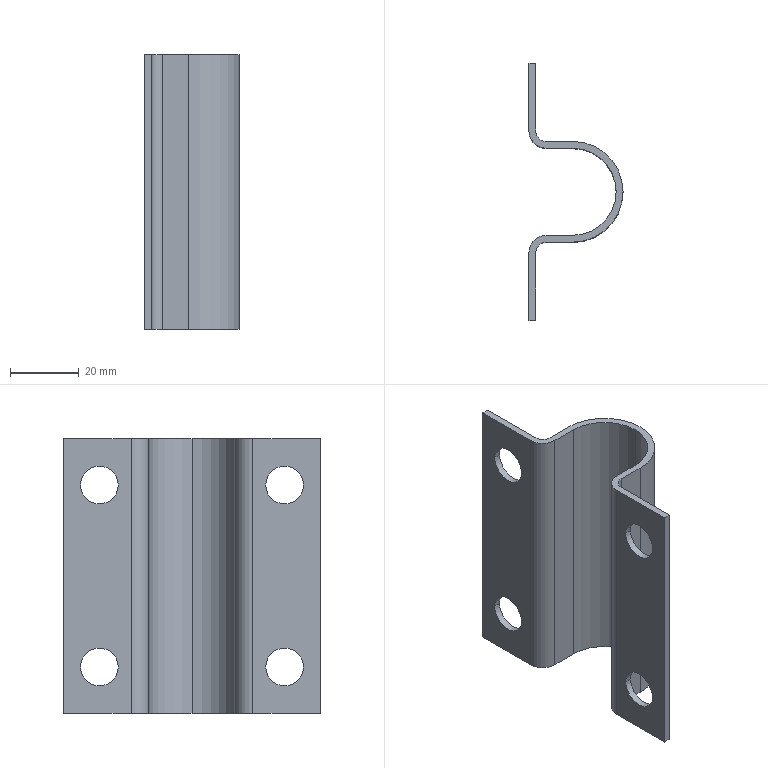Part | STEP file | 750031837 | 1 solid | 28 faces | box 27.4 x 75 x 80 mm | volume 16937 mm3 | cylinder 16 | plane 12 | commonest cylinder face diameters 11 x8 6 x2 10 x2 25.4 x2 29.4 x2
STEP:
#1=CARTESIAN_POINT('',(12.7,-14.7,0.));
#2=VERTEX_POINT('',#1);
#3=CARTESIAN_POINT('',(27.4,0.,0.));
#4=VERTEX_POINT('',#3);
#5=CARTESIAN_POINT('',(12.7,0.,0.));
#6=DIRECTION('',(0.,0.,1.));
#7=DIRECTION('',(1.,0.,0.));
#8=AXIS2_PLACEMENT_3D('',#5,#6,#7);
#9=CIRCLE('',#8,14.7);
#10=EDGE_CURVE('',#2,#4,#9,.T.);
#11=ORIENTED_EDGE('',*,*,#10,.T.);
#12=CARTESIAN_POINT('',(27.4,0.,80.));
#13=VERTEX_POINT('',#12);
#14=CARTESIAN_POINT('',(27.4,0.,0.));
#15=DIRECTION('',(0.,0.,1.));
#16=VECTOR('',#15,1000.);
#17=LINE('',#14,#16);
#18=EDGE_CURVE('',#4,#13,#17,.T.);
#19=ORIENTED_EDGE('',*,*,#18,.T.);
#20=CARTESIAN_POINT('',(12.7,-14.7,80.));
#21=VERTEX_POINT('',#20);
#22=CARTESIAN_POINT('',(12.7,0.,80.));
#23=DIRECTION('',(0.,0.,-1.));
#24=DIRECTION('',(1.,0.,0.));
#25=AXIS2_PLACEMENT_3D('',#22,#23,#24);
#26=CIRCLE('',#25,14.7);
#27=EDGE_CURVE('',#13,#21,#26,.T.);
#28=ORIENTED_EDGE('',*,*,#27,.T.);
#29=CARTESIAN_POINT('',(12.7,-14.7,0.));
#30=DIRECTION('',(0.,0.,-1.));
#31=VECTOR('',#30,1000.);
#32=LINE('',#29,#31);
#33=EDGE_CURVE('',#21,#2,#32,.T.);
#34=ORIENTED_EDGE('',*,*,#33,.T.);
#35=EDGE_LOOP('',(#11,#19,#28,#34));
#36=FACE_OUTER_BOUND('',#35,.T.);
#37=CARTESIAN_POINT('',(12.7,0.,0.));
#38=DIRECTION('',(0.,0.,1.));
#39=DIRECTION('',(1.,0.,0.));
#40=AXIS2_PLACEMENT_3D('',#37,#38,#39);
#41=CYLINDRICAL_SURFACE('',#40,14.7);
#42=ADVANCED_FACE('',(#36),#41,.T.);
#43=CARTESIAN_POINT('',(25.4,0.,0.));
#44=VERTEX_POINT('',#43);
#45=CARTESIAN_POINT('',(12.7,12.7,0.));
#46=VERTEX_POINT('',#45);
#47=CARTESIAN_POINT('',(12.7,0.,0.));
#48=DIRECTION('',(0.,0.,1.));
#49=DIRECTION('',(1.,0.,0.));
#50=AXIS2_PLACEMENT_3D('',#47,#48,#49);
#51=CIRCLE('',#50,12.7);
#52=EDGE_CURVE('',#44,#46,#51,.T.);
#53=ORIENTED_EDGE('',*,*,#52,.F.);
#54=CARTESIAN_POINT('',(25.4,0.,80.));
#55=VERTEX_POINT('',#54);
#56=CARTESIAN_POINT('',(25.4,0.,0.));
#57=DIRECTION('',(0.,0.,1.));
#58=VECTOR('',#57,1000.);
#59=LINE('',#56,#58);
#60=EDGE_CURVE('',#44,#55,#59,.T.);
#61=ORIENTED_EDGE('',*,*,#60,.T.);
#62=CARTESIAN_POINT('',(12.7,12.7,80.));
#63=VERTEX_POINT('',#62);
#64=CARTESIAN_POINT('',(12.7,0.,80.));
#65=DIRECTION('',(0.,0.,1.));
#66=DIRECTION('',(1.,0.,0.));
#67=AXIS2_PLACEMENT_3D('',#64,#65,#66);
#68=CIRCLE('',#67,12.7);
#69=EDGE_CURVE('',#55,#63,#68,.T.);
#70=ORIENTED_EDGE('',*,*,#69,.T.);
#71=CARTESIAN_POINT('',(12.7,12.7,0.));
#72=DIRECTION('',(0.,0.,1.));
#73=VECTOR('',#72,1000.);
#74=LINE('',#71,#73);
#75=EDGE_CURVE('',#46,#63,#74,.T.);
#76=ORIENTED_EDGE('',*,*,#75,.F.);
#77=EDGE_LOOP('',(#53,#61,#70,#76));
#78=FACE_OUTER_BOUND('',#77,.T.);
#79=CARTESIAN_POINT('',(12.7,0.,0.));
#80=DIRECTION('',(0.,0.,1.));
#81=DIRECTION('',(1.,0.,0.));
#82=AXIS2_PLACEMENT_3D('',#79,#80,#81);
#83=CYLINDRICAL_SURFACE('',#82,12.7);
#84=ADVANCED_FACE('',(#78),#83,.F.);
#85=CARTESIAN_POINT('',(2.,21.5,66.5));
#86=VERTEX_POINT('',#85);
#87=CARTESIAN_POINT('',(2.,32.5,66.5));
#88=VERTEX_POINT('',#87);
#89=CARTESIAN_POINT('',(2.,27.,66.5));
#90=DIRECTION('',(1.,0.,0.));
#91=DIRECTION('',(0.,-1.,0.));
#92=AXIS2_PLACEMENT_3D('',#89,#90,#91);
#93=CIRCLE('',#92,5.5);
#94=EDGE_CURVE('',#86,#88,#93,.T.);
#95=ORIENTED_EDGE('',*,*,#94,.T.);
#96=CARTESIAN_POINT('',(0.,32.5,66.5));
#97=VERTEX_POINT('',#96);
#98=CARTESIAN_POINT('',(113.03,32.5,66.5));
#99=DIRECTION('',(-1.,0.,0.));
#100=VECTOR('',#99,1000.);
#101=LINE('',#98,#100);
#102=EDGE_CURVE('',#88,#97,#101,.T.);
#103=ORIENTED_EDGE('',*,*,#102,.T.);
#104=CARTESIAN_POINT('',(0.,21.5,66.5));
#105=VERTEX_POINT('',#104);
#106=CARTESIAN_POINT('',(0.,27.,66.5));
#107=DIRECTION('',(1.,0.,0.));
#108=DIRECTION('',(0.,-1.,0.));
#109=AXIS2_PLACEMENT_3D('',#106,#107,#108);
#110=CIRCLE('',#109,5.5);
#111=EDGE_CURVE('',#105,#97,#110,.T.);
#112=ORIENTED_EDGE('',*,*,#111,.F.);
#113=CARTESIAN_POINT('',(113.03,21.5,66.5));
#114=DIRECTION('',(-1.,0.,0.));
#115=VECTOR('',#114,1000.);
#116=LINE('',#113,#115);
#117=EDGE_CURVE('',#86,#105,#116,.T.);
#118=ORIENTED_EDGE('',*,*,#117,.F.);
#119=EDGE_LOOP('',(#95,#103,#112,#118));
#120=FACE_OUTER_BOUND('',#119,.T.);
#121=CARTESIAN_POINT('',(113.03,27.,66.5));
#122=DIRECTION('',(-1.,0.,0.));
#123=DIRECTION('',(0.,-1.,0.));
#124=AXIS2_PLACEMENT_3D('',#121,#122,#123);
#125=CYLINDRICAL_SURFACE('',#124,5.5);
#126=ADVANCED_FACE('',(#120),#125,.F.);
#127=CARTESIAN_POINT('',(2.,21.5,13.5));
#128=VERTEX_POINT('',#127);
#129=CARTESIAN_POINT('',(2.,32.5,13.5));
#130=VERTEX_POINT('',#129);
#131=CARTESIAN_POINT('',(2.,27.,13.5));
#132=DIRECTION('',(1.,0.,0.));
#133=DIRECTION('',(0.,-1.,0.));
#134=AXIS2_PLACEMENT_3D('',#131,#132,#133);
#135=CIRCLE('',#134,5.5);
#136=EDGE_CURVE('',#128,#130,#135,.T.);
#137=ORIENTED_EDGE('',*,*,#136,.T.);
#138=CARTESIAN_POINT('',(0.,32.5,13.5));
#139=VERTEX_POINT('',#138);
#140=CARTESIAN_POINT('',(113.03,32.5,13.5));
#141=DIRECTION('',(-1.,0.,0.));
#142=VECTOR('',#141,1000.);
#143=LINE('',#140,#142);
#144=EDGE_CURVE('',#130,#139,#143,.T.);
#145=ORIENTED_EDGE('',*,*,#144,.T.);
#146=CARTESIAN_POINT('',(0.,21.5,13.5));
#147=VERTEX_POINT('',#146);
#148=CARTESIAN_POINT('',(0.,27.,13.5));
#149=DIRECTION('',(1.,0.,0.));
#150=DIRECTION('',(0.,-1.,0.));
#151=AXIS2_PLACEMENT_3D('',#148,#149,#150);
#152=CIRCLE('',#151,5.5);
#153=EDGE_CURVE('',#147,#139,#152,.T.);
#154=ORIENTED_EDGE('',*,*,#153,.F.);
#155=CARTESIAN_POINT('',(113.03,21.5,13.5));
#156=DIRECTION('',(-1.,0.,0.));
#157=VECTOR('',#156,1000.);
#158=LINE('',#155,#157);
#159=EDGE_CURVE('',#128,#147,#158,.T.);
#160=ORIENTED_EDGE('',*,*,#159,.F.);
#161=EDGE_LOOP('',(#137,#145,#154,#160));
#162=FACE_OUTER_BOUND('',#161,.T.);
#163=CARTESIAN_POINT('',(113.03,27.,13.5));
#164=DIRECTION('',(-1.,0.,0.));
#165=DIRECTION('',(0.,-1.,0.));
#166=AXIS2_PLACEMENT_3D('',#163,#164,#165);
#167=CYLINDRICAL_SURFACE('',#166,5.5);
#168=ADVANCED_FACE('',(#162),#167,.F.);
#169=CARTESIAN_POINT('',(2.,-32.5,66.5));
#170=VERTEX_POINT('',#169);
#171=CARTESIAN_POINT('',(2.,-21.5,66.5));
#172=VERTEX_POINT('',#171);
#173=CARTESIAN_POINT('',(2.,-27.,66.5));
#174=DIRECTION('',(1.,0.,0.));
#175=DIRECTION('',(0.,-1.,0.));
#176=AXIS2_PLACEMENT_3D('',#173,#174,#175);
#177=CIRCLE('',#176,5.5);
#178=EDGE_CURVE('',#170,#172,#177,.T.);
#179=ORIENTED_EDGE('',*,*,#178,.T.);
#180=CARTESIAN_POINT('',(0.,-21.5,66.5));
#181=VERTEX_POINT('',#180);
#182=CARTESIAN_POINT('',(113.03,-21.5,66.5));
#183=DIRECTION('',(-1.,0.,0.));
#184=VECTOR('',#183,1000.);
#185=LINE('',#182,#184);
#186=EDGE_CURVE('',#172,#181,#185,.T.);
#187=ORIENTED_EDGE('',*,*,#186,.T.);
#188=CARTESIAN_POINT('',(0.,-32.5,66.5));
#189=VERTEX_POINT('',#188);
#190=CARTESIAN_POINT('',(0.,-27.,66.5));
#191=DIRECTION('',(1.,0.,0.));
#192=DIRECTION('',(0.,-1.,0.));
#193=AXIS2_PLACEMENT_3D('',#190,#191,#192);
#194=CIRCLE('',#193,5.5);
#195=EDGE_CURVE('',#189,#181,#194,.T.);
#196=ORIENTED_EDGE('',*,*,#195,.F.);
#197=CARTESIAN_POINT('',(113.03,-32.5,66.5));
#198=DIRECTION('',(-1.,0.,0.));
#199=VECTOR('',#198,1000.);
#200=LINE('',#197,#199);
#201=EDGE_CURVE('',#170,#189,#200,.T.);
#202=ORIENTED_EDGE('',*,*,#201,.F.);
#203=EDGE_LOOP('',(#179,#187,#196,#202));
#204=FACE_OUTER_BOUND('',#203,.T.);
#205=CARTESIAN_POINT('',(113.03,-27.,66.5));
#206=DIRECTION('',(-1.,0.,0.));
#207=DIRECTION('',(0.,-1.,0.));
#208=AXIS2_PLACEMENT_3D('',#205,#206,#207);
#209=CYLINDRICAL_SURFACE('',#208,5.5);
#210=ADVANCED_FACE('',(#204),#209,.F.);
#211=CARTESIAN_POINT('',(2.,-32.5,13.5));
#212=VERTEX_POINT('',#211);
#213=CARTESIAN_POINT('',(2.,-21.5,13.5));
#214=VERTEX_POINT('',#213);
#215=CARTESIAN_POINT('',(2.,-27.,13.5));
#216=DIRECTION('',(1.,0.,0.));
#217=DIRECTION('',(0.,-1.,0.));
#218=AXIS2_PLACEMENT_3D('',#215,#216,#217);
#219=CIRCLE('',#218,5.5);
#220=EDGE_CURVE('',#212,#214,#219,.T.);
#221=ORIENTED_EDGE('',*,*,#220,.T.);
#222=CARTESIAN_POINT('',(0.,-21.5,13.5));
#223=VERTEX_POINT('',#222);
#224=CARTESIAN_POINT('',(113.03,-21.5,13.5));
#225=DIRECTION('',(-1.,0.,0.));
#226=VECTOR('',#225,1000.);
#227=LINE('',#224,#226);
#228=EDGE_CURVE('',#214,#223,#227,.T.);
#229=ORIENTED_EDGE('',*,*,#228,.T.);
#230=CARTESIAN_POINT('',(0.,-32.5,13.5));
#231=VERTEX_POINT('',#230);
#232=CARTESIAN_POINT('',(0.,-27.,13.5));
#233=DIRECTION('',(1.,0.,0.));
#234=DIRECTION('',(0.,-1.,0.));
#235=AXIS2_PLACEMENT_3D('',#232,#233,#234);
#236=CIRCLE('',#235,5.5);
#237=EDGE_CURVE('',#231,#223,#236,.T.);
#238=ORIENTED_EDGE('',*,*,#237,.F.);
#239=CARTESIAN_POINT('',(113.03,-32.5,13.5));
#240=DIRECTION('',(-1.,0.,0.));
#241=VECTOR('',#240,1000.);
#242=LINE('',#239,#241);
#243=EDGE_CURVE('',#212,#231,#242,.T.);
#244=ORIENTED_EDGE('',*,*,#243,.F.);
#245=EDGE_LOOP('',(#221,#229,#238,#244));
#246=FACE_OUTER_BOUND('',#245,.T.);
#247=CARTESIAN_POINT('',(113.03,-27.,13.5));
#248=DIRECTION('',(-1.,0.,0.));
#249=DIRECTION('',(0.,-1.,0.));
#250=AXIS2_PLACEMENT_3D('',#247,#248,#249);
#251=CYLINDRICAL_SURFACE('',#250,5.5);
#252=ADVANCED_FACE('',(#246),#251,.F.);
#253=ORIENTED_EDGE('',*,*,#18,.F.);
#254=CARTESIAN_POINT('',(12.7,14.7,0.));
#255=VERTEX_POINT('',#254);
#256=CARTESIAN_POINT('',(12.7,0.,0.));
#257=DIRECTION('',(0.,0.,1.));
#258=DIRECTION('',(1.,0.,0.));
#259=AXIS2_PLACEMENT_3D('',#256,#257,#258);
#260=CIRCLE('',#259,14.7);
#261=EDGE_CURVE('',#4,#255,#260,.T.);
#262=ORIENTED_EDGE('',*,*,#261,.T.);
#263=CARTESIAN_POINT('',(12.7,14.7,80.));
#264=VERTEX_POINT('',#263);
#265=CARTESIAN_POINT('',(12.7,14.7,0.));
#266=DIRECTION('',(0.,0.,1.));
#267=VECTOR('',#266,1000.);
#268=LINE('',#265,#267);
#269=EDGE_CURVE('',#255,#264,#268,.T.);
#270=ORIENTED_EDGE('',*,*,#269,.T.);
#271=CARTESIAN_POINT('',(12.7,0.,80.));
#272=DIRECTION('',(0.,0.,-1.));
#273=DIRECTION('',(1.,0.,0.));
#274=AXIS2_PLACEMENT_3D('',#271,#272,#273);
#275=CIRCLE('',#274,14.7);
#276=EDGE_CURVE('',#264,#13,#275,.T.);
#277=ORIENTED_EDGE('',*,*,#276,.T.);
#278=EDGE_LOOP('',(#253,#262,#270,#277));
#279=FACE_OUTER_BOUND('',#278,.T.);
#280=CARTESIAN_POINT('',(12.7,0.,0.));
#281=DIRECTION('',(0.,0.,1.));
#282=DIRECTION('',(1.,0.,0.));
#283=AXIS2_PLACEMENT_3D('',#280,#281,#282);
#284=CYLINDRICAL_SURFACE('',#283,14.7);
#285=ADVANCED_FACE('',(#279),#284,.T.);
#286=ORIENTED_EDGE('',*,*,#269,.F.);
#287=CARTESIAN_POINT('',(5.,14.7,0.));
#288=VERTEX_POINT('',#287);
#289=CARTESIAN_POINT('',(5.,14.7,0.));
#290=DIRECTION('',(1.,0.,0.));
#291=VECTOR('',#290,1000.);
#292=LINE('',#289,#291);
#293=EDGE_CURVE('',#288,#255,#292,.T.);
#294=ORIENTED_EDGE('',*,*,#293,.F.);
#295=CARTESIAN_POINT('',(5.,14.7,80.));
#296=VERTEX_POINT('',#295);
#297=CARTESIAN_POINT('',(5.,14.7,0.));
#298=DIRECTION('',(0.,0.,-1.));
#299=VECTOR('',#298,1000.);
#300=LINE('',#297,#299);
#301=EDGE_CURVE('',#296,#288,#300,.T.);
#302=ORIENTED_EDGE('',*,*,#301,.F.);
#303=CARTESIAN_POINT('',(5.,14.7,80.));
#304=DIRECTION('',(-1.,0.,0.));
#305=VECTOR('',#304,1000.);
#306=LINE('',#303,#305);
#307=EDGE_CURVE('',#264,#296,#306,.T.);
#308=ORIENTED_EDGE('',*,*,#307,.F.);
#309=EDGE_LOOP('',(#286,#294,#302,#308));
#310=FACE_OUTER_BOUND('',#309,.T.);
#311=CARTESIAN_POINT('',(5.,14.7,0.));
#312=DIRECTION('',(0.,-1.,0.));
#313=DIRECTION('',(0.,0.,-1.));
#314=AXIS2_PLACEMENT_3D('',#311,#312,#313);
#315=PLANE('',#314);
#316=ADVANCED_FACE('',(#310),#315,.F.);
#317=CARTESIAN_POINT('',(0.,17.7,0.));
#318=VERTEX_POINT('',#317);
#319=CARTESIAN_POINT('',(0.,37.5,0.));
#320=VERTEX_POINT('',#319);
#321=CARTESIAN_POINT('',(0.,37.5,0.));
#322=DIRECTION('',(0.,1.,0.));
#323=VECTOR('',#322,1000.);
#324=LINE('',#321,#323);
#325=EDGE_CURVE('',#318,#320,#324,.T.);
#326=ORIENTED_EDGE('',*,*,#325,.T.);
#327=CARTESIAN_POINT('',(2.,37.5,0.));
#328=VERTEX_POINT('',#327);
#329=CARTESIAN_POINT('',(0.,37.5,0.));
#330=DIRECTION('',(1.,0.,0.));
#331=VECTOR('',#330,1000.);
#332=LINE('',#329,#331);
#333=EDGE_CURVE('',#320,#328,#332,.T.);
#334=ORIENTED_EDGE('',*,*,#333,.T.);
#335=CARTESIAN_POINT('',(2.,17.7,0.));
#336=VERTEX_POINT('',#335);
#337=CARTESIAN_POINT('',(2.,37.5,0.));
#338=DIRECTION('',(0.,-1.,0.));
#339=VECTOR('',#338,1000.);
#340=LINE('',#337,#339);
#341=EDGE_CURVE('',#328,#336,#340,.T.);
#342=ORIENTED_EDGE('',*,*,#341,.T.);
#343=CARTESIAN_POINT('',(5.,17.7,0.));
#344=DIRECTION('',(0.,0.,1.));
#345=DIRECTION('',(1.,0.,0.));
#346=AXIS2_PLACEMENT_3D('',#343,#344,#345);
#347=CIRCLE('',#346,3.);
#348=EDGE_CURVE('',#336,#288,#347,.T.);
#349=ORIENTED_EDGE('',*,*,#348,.T.);
#350=ORIENTED_EDGE('',*,*,#293,.T.);
#351=ORIENTED_EDGE('',*,*,#261,.F.);
#352=ORIENTED_EDGE('',*,*,#10,.F.);
#353=CARTESIAN_POINT('',(5.,-14.7,0.));
#354=VERTEX_POINT('',#353);
#355=CARTESIAN_POINT('',(0.,-14.7,0.));
#356=DIRECTION('',(-1.,0.,0.));
#357=VECTOR('',#356,1000.);
#358=LINE('',#355,#357);
#359=EDGE_CURVE('',#2,#354,#358,.T.);
#360=ORIENTED_EDGE('',*,*,#359,.T.);
#361=CARTESIAN_POINT('',(2.,-17.7,0.));
#362=VERTEX_POINT('',#361);
#363=CARTESIAN_POINT('',(5.,-17.7,0.));
#364=DIRECTION('',(0.,0.,1.));
#365=DIRECTION('',(1.,0.,0.));
#366=AXIS2_PLACEMENT_3D('',#363,#364,#365);
#367=CIRCLE('',#366,3.);
#368=EDGE_CURVE('',#354,#362,#367,.T.);
#369=ORIENTED_EDGE('',*,*,#368,.T.);
#370=CARTESIAN_POINT('',(2.,-37.5,0.));
#371=VERTEX_POINT('',#370);
#372=CARTESIAN_POINT('',(2.,37.5,0.));
#373=DIRECTION('',(0.,-1.,0.));
#374=VECTOR('',#373,1000.);
#375=LINE('',#372,#374);
#376=EDGE_CURVE('',#362,#371,#375,.T.);
#377=ORIENTED_EDGE('',*,*,#376,.T.);
#378=CARTESIAN_POINT('',(0.,-37.5,0.));
#379=VERTEX_POINT('',#378);
#380=CARTESIAN_POINT('',(0.,-37.5,0.));
#381=DIRECTION('',(-1.,0.,0.));
#382=VECTOR('',#381,1000.);
#383=LINE('',#380,#382);
#384=EDGE_CURVE('',#371,#379,#383,.T.);
#385=ORIENTED_EDGE('',*,*,#384,.T.);
#386=CARTESIAN_POINT('',(0.,-17.7,0.));
#387=VERTEX_POINT('',#386);
#388=CARTESIAN_POINT('',(0.,37.5,0.));
#389=DIRECTION('',(0.,1.,0.));
#390=VECTOR('',#389,1000.);
#391=LINE('',#388,#390);
#392=EDGE_CURVE('',#379,#387,#391,.T.);
#393=ORIENTED_EDGE('',*,*,#392,.T.);
#394=CARTESIAN_POINT('',(5.,-12.7,0.));
#395=VERTEX_POINT('',#394);
#396=CARTESIAN_POINT('',(5.,-17.7,0.));
#397=DIRECTION('',(0.,0.,-1.));
#398=DIRECTION('',(1.,0.,0.));
#399=AXIS2_PLACEMENT_3D('',#396,#397,#398);
#400=CIRCLE('',#399,5.);
#401=EDGE_CURVE('',#387,#395,#400,.T.);
#402=ORIENTED_EDGE('',*,*,#401,.T.);
#403=CARTESIAN_POINT('',(12.7,-12.7,0.));
#404=VERTEX_POINT('',#403);
#405=CARTESIAN_POINT('',(0.,-12.7,0.));
#406=DIRECTION('',(1.,0.,0.));
#407=VECTOR('',#406,1000.);
#408=LINE('',#405,#407);
#409=EDGE_CURVE('',#395,#404,#408,.T.);
#410=ORIENTED_EDGE('',*,*,#409,.T.);
#411=CARTESIAN_POINT('',(12.7,0.,0.));
#412=DIRECTION('',(0.,0.,1.));
#413=DIRECTION('',(1.,0.,0.));
#414=AXIS2_PLACEMENT_3D('',#411,#412,#413);
#415=CIRCLE('',#414,12.7);
#416=EDGE_CURVE('',#404,#44,#415,.T.);
#417=ORIENTED_EDGE('',*,*,#416,.T.);
#418=ORIENTED_EDGE('',*,*,#52,.T.);
#419=CARTESIAN_POINT('',(5.,12.7,0.));
#420=VERTEX_POINT('',#419);
#421=CARTESIAN_POINT('',(0.,12.7,0.));
#422=DIRECTION('',(-1.,0.,0.));
#423=VECTOR('',#422,1000.);
#424=LINE('',#421,#423);
#425=EDGE_CURVE('',#46,#420,#424,.T.);
#426=ORIENTED_EDGE('',*,*,#425,.T.);
#427=CARTESIAN_POINT('',(5.,17.7,0.));
#428=DIRECTION('',(0.,0.,-1.));
#429=DIRECTION('',(1.,0.,0.));
#430=AXIS2_PLACEMENT_3D('',#427,#428,#429);
#431=CIRCLE('',#430,5.);
#432=EDGE_CURVE('',#420,#318,#431,.T.);
#433=ORIENTED_EDGE('',*,*,#432,.T.);
#434=EDGE_LOOP('',(#326,#334,#342,#349,#350,#351,#352,#360,#369,#377,#385,#393,#402,#410,#417,#418,#426,#433));
#435=FACE_OUTER_BOUND('',#434,.T.);
#436=CARTESIAN_POINT('',(0.,37.5,0.));
#437=DIRECTION('',(0.,0.,-1.));
#438=DIRECTION('',(-1.,0.,0.));
#439=AXIS2_PLACEMENT_3D('',#436,#437,#438);
#440=PLANE('',#439);
#441=ADVANCED_FACE('',(#435),#440,.T.);
#442=CARTESIAN_POINT('',(5.,-14.7,80.));
#443=VERTEX_POINT('',#442);
#444=CARTESIAN_POINT('',(5.,-14.7,0.));
#445=DIRECTION('',(0.,0.,1.));
#446=VECTOR('',#445,1000.);
#447=LINE('',#444,#446);
#448=EDGE_CURVE('',#354,#443,#447,.T.);
#449=ORIENTED_EDGE('',*,*,#448,.F.);
#450=ORIENTED_EDGE('',*,*,#359,.F.);
#451=ORIENTED_EDGE('',*,*,#33,.F.);
#452=CARTESIAN_POINT('',(12.7,-14.7,80.));
#453=DIRECTION('',(1.,0.,0.));
#454=VECTOR('',#453,1000.);
#455=LINE('',#452,#454);
#456=EDGE_CURVE('',#443,#21,#455,.T.);
#457=ORIENTED_EDGE('',*,*,#456,.F.);
#458=EDGE_LOOP('',(#449,#450,#451,#457));
#459=FACE_OUTER_BOUND('',#458,.T.);
#460=CARTESIAN_POINT('',(12.7,-14.7,0.));
#461=DIRECTION('',(0.,1.,0.));
#462=DIRECTION('',(0.,0.,1.));
#463=AXIS2_PLACEMENT_3D('',#460,#461,#462);
#464=PLANE('',#463);
#465=ADVANCED_FACE('',(#459),#464,.F.);
#466=CARTESIAN_POINT('',(5.,12.7,80.));
#467=VERTEX_POINT('',#466);
#468=CARTESIAN_POINT('',(5.,12.7,80.));
#469=DIRECTION('',(-1.,0.,0.));
#470=VECTOR('',#469,1000.);
#471=LINE('',#468,#470);
#472=EDGE_CURVE('',#63,#467,#471,.T.);
#473=ORIENTED_EDGE('',*,*,#472,.F.);
#474=ORIENTED_EDGE('',*,*,#69,.F.);
#475=CARTESIAN_POINT('',(12.7,-12.7,80.));
#476=VERTEX_POINT('',#475);
#477=CARTESIAN_POINT('',(12.7,0.,80.));
#478=DIRECTION('',(0.,0.,1.));
#479=DIRECTION('',(1.,0.,0.));
#480=AXIS2_PLACEMENT_3D('',#477,#478,#479);
#481=CIRCLE('',#480,12.7);
#482=EDGE_CURVE('',#476,#55,#481,.T.);
#483=ORIENTED_EDGE('',*,*,#482,.F.);
#484=CARTESIAN_POINT('',(5.,-12.7,80.));
#485=VERTEX_POINT('',#484);
#486=CARTESIAN_POINT('',(5.,-12.7,80.));
#487=DIRECTION('',(1.,0.,0.));
#488=VECTOR('',#487,1000.);
#489=LINE('',#486,#488);
#490=EDGE_CURVE('',#485,#476,#489,.T.);
#491=ORIENTED_EDGE('',*,*,#490,.F.);
#492=CARTESIAN_POINT('',(0.,-17.7,80.));
#493=VERTEX_POINT('',#492);
#494=CARTESIAN_POINT('',(5.,-17.7,80.));
#495=DIRECTION('',(0.,0.,-1.));
#496=DIRECTION('',(1.,0.,0.));
#497=AXIS2_PLACEMENT_3D('',#494,#495,#496);
#498=CIRCLE('',#497,5.);
#499=EDGE_CURVE('',#493,#485,#498,.T.);
#500=ORIENTED_EDGE('',*,*,#499,.F.);
#501=CARTESIAN_POINT('',(0.,-37.5,80.));
#502=VERTEX_POINT('',#501);
#503=CARTESIAN_POINT('',(0.,17.7,80.));
#504=DIRECTION('',(0.,1.,0.));
#505=VECTOR('',#504,1000.);
#506=LINE('',#503,#505);
#507=EDGE_CURVE('',#502,#493,#506,.T.);
#508=ORIENTED_EDGE('',*,*,#507,.F.);
#509=CARTESIAN_POINT('',(2.,-37.5,80.));
#510=VERTEX_POINT('',#509);
#511=CARTESIAN_POINT('',(5.,-37.5,80.));
#512=DIRECTION('',(-1.,0.,0.));
#513=VECTOR('',#512,1000.);
#514=LINE('',#511,#513);
#515=EDGE_CURVE('',#510,#502,#514,.T.);
#516=ORIENTED_EDGE('',*,*,#515,.F.);
#517=CARTESIAN_POINT('',(2.,-17.7,80.));
#518=VERTEX_POINT('',#517);
#519=CARTESIAN_POINT('',(2.,17.7,80.));
#520=DIRECTION('',(0.,-1.,0.));
#521=VECTOR('',#520,1000.);
#522=LINE('',#519,#521);
#523=EDGE_CURVE('',#518,#510,#522,.T.);
#524=ORIENTED_EDGE('',*,*,#523,.F.);
#525=CARTESIAN_POINT('',(5.,-17.7,80.));
#526=DIRECTION('',(0.,0.,1.));
#527=DIRECTION('',(1.,0.,0.));
#528=AXIS2_PLACEMENT_3D('',#525,#526,#527);
#529=CIRCLE('',#528,3.);
#530=EDGE_CURVE('',#443,#518,#529,.T.);
#531=ORIENTED_EDGE('',*,*,#530,.F.);
#532=ORIENTED_EDGE('',*,*,#456,.T.);
#533=ORIENTED_EDGE('',*,*,#27,.F.);
#534=ORIENTED_EDGE('',*,*,#276,.F.);
#535=ORIENTED_EDGE('',*,*,#307,.T.);
#536=CARTESIAN_POINT('',(2.,17.7,80.));
#537=VERTEX_POINT('',#536);
#538=CARTESIAN_POINT('',(5.,17.7,80.));
#539=DIRECTION('',(0.,0.,1.));
#540=DIRECTION('',(1.,0.,0.));
#541=AXIS2_PLACEMENT_3D('',#538,#539,#540);
#542=CIRCLE('',#541,3.);
#543=EDGE_CURVE('',#537,#296,#542,.T.);
#544=ORIENTED_EDGE('',*,*,#543,.F.);
#545=CARTESIAN_POINT('',(2.,37.5,80.));
#546=VERTEX_POINT('',#545);
#547=CARTESIAN_POINT('',(2.,17.7,80.));
#548=DIRECTION('',(0.,-1.,0.));
#549=VECTOR('',#548,1000.);
#550=LINE('',#547,#549);
#551=EDGE_CURVE('',#546,#537,#550,.T.);
#552=ORIENTED_EDGE('',*,*,#551,.F.);
#553=CARTESIAN_POINT('',(0.,37.5,80.));
#554=VERTEX_POINT('',#553);
#555=CARTESIAN_POINT('',(5.,37.5,80.));
#556=DIRECTION('',(1.,0.,0.));
#557=VECTOR('',#556,1000.);
#558=LINE('',#555,#557);
#559=EDGE_CURVE('',#554,#546,#558,.T.);
#560=ORIENTED_EDGE('',*,*,#559,.F.);
#561=CARTESIAN_POINT('',(0.,17.7,80.));
#562=VERTEX_POINT('',#561);
#563=CARTESIAN_POINT('',(0.,17.7,80.));
#564=DIRECTION('',(0.,1.,0.));
#565=VECTOR('',#564,1000.);
#566=LINE('',#563,#565);
#567=EDGE_CURVE('',#562,#554,#566,.T.);
#568=ORIENTED_EDGE('',*,*,#567,.F.);
#569=CARTESIAN_POINT('',(5.,17.7,80.));
#570=DIRECTION('',(0.,0.,-1.));
#571=DIRECTION('',(1.,0.,0.));
#572=AXIS2_PLACEMENT_3D('',#569,#570,#571);
#573=CIRCLE('',#572,5.);
#574=EDGE_CURVE('',#467,#562,#573,.T.);
#575=ORIENTED_EDGE('',*,*,#574,.F.);
#576=EDGE_LOOP('',(#473,#474,#483,#491,#500,#508,#516,#524,#531,#532,#533,#534,#535,#544,#552,#560,#568,#575));
#577=FACE_OUTER_BOUND('',#576,.T.);
#578=CARTESIAN_POINT('',(5.,17.7,80.));
#579=DIRECTION('',(0.,0.,-1.));
#580=DIRECTION('',(-1.,0.,0.));
#581=AXIS2_PLACEMENT_3D('',#578,#579,#580);
#582=PLANE('',#581);
#583=ADVANCED_FACE('',(#577),#582,.F.);
#584=ORIENTED_EDGE('',*,*,#301,.T.);
#585=ORIENTED_EDGE('',*,*,#348,.F.);
#586=CARTESIAN_POINT('',(2.,17.7,0.));
#587=DIRECTION('',(0.,0.,-1.));
#588=VECTOR('',#587,1000.);
#589=LINE('',#586,#588);
#590=EDGE_CURVE('',#537,#336,#589,.T.);
#591=ORIENTED_EDGE('',*,*,#590,.F.);
#592=ORIENTED_EDGE('',*,*,#543,.T.);
#593=EDGE_LOOP('',(#584,#585,#591,#592));
#594=FACE_OUTER_BOUND('',#593,.T.);
#595=CARTESIAN_POINT('',(5.,17.7,0.));
#596=DIRECTION('',(0.,0.,1.));
#597=DIRECTION('',(1.,0.,0.));
#598=AXIS2_PLACEMENT_3D('',#595,#596,#597);
#599=CYLINDRICAL_SURFACE('',#598,3.);
#600=ADVANCED_FACE('',(#594),#599,.F.);
#601=CARTESIAN_POINT('',(0.,37.5,0.));
#602=DIRECTION('',(0.,0.,-1.));
#603=VECTOR('',#602,1000.);
#604=LINE('',#601,#603);
#605=EDGE_CURVE('',#554,#320,#604,.T.);
#606=ORIENTED_EDGE('',*,*,#605,.F.);
#607=ORIENTED_EDGE('',*,*,#559,.T.);
#608=CARTESIAN_POINT('',(2.,37.5,0.));
#609=DIRECTION('',(0.,0.,1.));
#610=VECTOR('',#609,1000.);
#611=LINE('',#608,#610);
#612=EDGE_CURVE('',#328,#546,#611,.T.);
#613=ORIENTED_EDGE('',*,*,#612,.F.);
#614=ORIENTED_EDGE('',*,*,#333,.F.);
#615=EDGE_LOOP('',(#606,#607,#613,#614));
#616=FACE_OUTER_BOUND('',#615,.T.);
#617=CARTESIAN_POINT('',(0.,37.5,0.));
#618=DIRECTION('',(0.,-1.,0.));
#619=DIRECTION('',(0.,0.,-1.));
#620=AXIS2_PLACEMENT_3D('',#617,#618,#619);
#621=PLANE('',#620);
#622=ADVANCED_FACE('',(#616),#621,.F.);
#623=ORIENTED_EDGE('',*,*,#325,.F.);
#624=CARTESIAN_POINT('',(0.,17.7,0.));
#625=DIRECTION('',(0.,0.,1.));
#626=VECTOR('',#625,1000.);
#627=LINE('',#624,#626);
#628=EDGE_CURVE('',#318,#562,#627,.T.);
#629=ORIENTED_EDGE('',*,*,#628,.T.);
#630=ORIENTED_EDGE('',*,*,#567,.T.);
#631=ORIENTED_EDGE('',*,*,#605,.T.);
#632=EDGE_LOOP('',(#623,#629,#630,#631));
#633=FACE_OUTER_BOUND('',#632,.T.);
#634=ORIENTED_EDGE('',*,*,#111,.T.);
#635=CARTESIAN_POINT('',(0.,27.,66.5));
#636=DIRECTION('',(1.,0.,0.));
#637=DIRECTION('',(0.,-1.,0.));
#638=AXIS2_PLACEMENT_3D('',#635,#636,#637);
#639=CIRCLE('',#638,5.5);
#640=EDGE_CURVE('',#97,#105,#639,.T.);
#641=ORIENTED_EDGE('',*,*,#640,.T.);
#642=EDGE_LOOP('',(#634,#641));
#643=FACE_BOUND('',#642,.T.);
#644=ORIENTED_EDGE('',*,*,#153,.T.);
#645=CARTESIAN_POINT('',(0.,27.,13.5));
#646=DIRECTION('',(1.,0.,0.));
#647=DIRECTION('',(0.,-1.,0.));
#648=AXIS2_PLACEMENT_3D('',#645,#646,#647);
#649=CIRCLE('',#648,5.5);
#650=EDGE_CURVE('',#139,#147,#649,.T.);
#651=ORIENTED_EDGE('',*,*,#650,.T.);
#652=EDGE_LOOP('',(#644,#651));
#653=FACE_BOUND('',#652,.T.);
#654=CARTESIAN_POINT('',(0.,37.5,0.));
#655=DIRECTION('',(-1.,0.,0.));
#656=DIRECTION('',(0.,0.,1.));
#657=AXIS2_PLACEMENT_3D('',#654,#655,#656);
#658=PLANE('',#657);
#659=ADVANCED_FACE('',(#633,#643,#653),#658,.T.);
#660=ORIENTED_EDGE('',*,*,#432,.F.);
#661=CARTESIAN_POINT('',(5.,12.7,0.));
#662=DIRECTION('',(0.,0.,1.));
#663=VECTOR('',#662,1000.);
#664=LINE('',#661,#663);
#665=EDGE_CURVE('',#420,#467,#664,.T.);
#666=ORIENTED_EDGE('',*,*,#665,.T.);
#667=ORIENTED_EDGE('',*,*,#574,.T.);
#668=ORIENTED_EDGE('',*,*,#628,.F.);
#669=EDGE_LOOP('',(#660,#666,#667,#668));
#670=FACE_OUTER_BOUND('',#669,.T.);
#671=CARTESIAN_POINT('',(5.,17.7,0.));
#672=DIRECTION('',(0.,0.,1.));
#673=DIRECTION('',(1.,0.,0.));
#674=AXIS2_PLACEMENT_3D('',#671,#672,#673);
#675=CYLINDRICAL_SURFACE('',#674,5.);
#676=ADVANCED_FACE('',(#670),#675,.T.);
#677=ORIENTED_EDGE('',*,*,#425,.F.);
#678=ORIENTED_EDGE('',*,*,#75,.T.);
#679=ORIENTED_EDGE('',*,*,#472,.T.);
#680=ORIENTED_EDGE('',*,*,#665,.F.);
#681=EDGE_LOOP('',(#677,#678,#679,#680));
#682=FACE_OUTER_BOUND('',#681,.T.);
#683=CARTESIAN_POINT('',(5.,12.7,0.));
#684=DIRECTION('',(0.,-1.,0.));
#685=DIRECTION('',(0.,0.,-1.));
#686=AXIS2_PLACEMENT_3D('',#683,#684,#685);
#687=PLANE('',#686);
#688=ADVANCED_FACE('',(#682),#687,.T.);
#689=ORIENTED_EDGE('',*,*,#60,.F.);
#690=ORIENTED_EDGE('',*,*,#416,.F.);
#691=CARTESIAN_POINT('',(12.7,-12.7,0.));
#692=DIRECTION('',(0.,0.,-1.));
#693=VECTOR('',#692,1000.);
#694=LINE('',#691,#693);
#695=EDGE_CURVE('',#476,#404,#694,.T.);
#696=ORIENTED_EDGE('',*,*,#695,.F.);
#697=ORIENTED_EDGE('',*,*,#482,.T.);
#698=EDGE_LOOP('',(#689,#690,#696,#697));
#699=FACE_OUTER_BOUND('',#698,.T.);
#700=CARTESIAN_POINT('',(12.7,0.,0.));
#701=DIRECTION('',(0.,0.,1.));
#702=DIRECTION('',(1.,0.,0.));
#703=AXIS2_PLACEMENT_3D('',#700,#701,#702);
#704=CYLINDRICAL_SURFACE('',#703,12.7);
#705=ADVANCED_FACE('',(#699),#704,.F.);
#706=ORIENTED_EDGE('',*,*,#409,.F.);
#707=CARTESIAN_POINT('',(5.,-12.7,0.));
#708=DIRECTION('',(0.,0.,1.));
#709=VECTOR('',#708,1000.);
#710=LINE('',#707,#709);
#711=EDGE_CURVE('',#395,#485,#710,.T.);
#712=ORIENTED_EDGE('',*,*,#711,.T.);
#713=ORIENTED_EDGE('',*,*,#490,.T.);
#714=ORIENTED_EDGE('',*,*,#695,.T.);
#715=EDGE_LOOP('',(#706,#712,#713,#714));
#716=FACE_OUTER_BOUND('',#715,.T.);
#717=CARTESIAN_POINT('',(12.7,-12.7,0.));
#718=DIRECTION('',(0.,1.,0.));
#719=DIRECTION('',(0.,0.,1.));
#720=AXIS2_PLACEMENT_3D('',#717,#718,#719);
#721=PLANE('',#720);
#722=ADVANCED_FACE('',(#716),#721,.T.);
#723=ORIENTED_EDGE('',*,*,#401,.F.);
#724=CARTESIAN_POINT('',(0.,-17.7,0.));
#725=DIRECTION('',(0.,0.,1.));
#726=VECTOR('',#725,1000.);
#727=LINE('',#724,#726);
#728=EDGE_CURVE('',#387,#493,#727,.T.);
#729=ORIENTED_EDGE('',*,*,#728,.T.);
#730=ORIENTED_EDGE('',*,*,#499,.T.);
#731=ORIENTED_EDGE('',*,*,#711,.F.);
#732=EDGE_LOOP('',(#723,#729,#730,#731));
#733=FACE_OUTER_BOUND('',#732,.T.);
#734=CARTESIAN_POINT('',(5.,-17.7,0.));
#735=DIRECTION('',(0.,0.,1.));
#736=DIRECTION('',(1.,0.,0.));
#737=AXIS2_PLACEMENT_3D('',#734,#735,#736);
#738=CYLINDRICAL_SURFACE('',#737,5.);
#739=ADVANCED_FACE('',(#733),#738,.T.);
#740=ORIENTED_EDGE('',*,*,#392,.F.);
#741=CARTESIAN_POINT('',(0.,-37.5,0.));
#742=DIRECTION('',(0.,0.,1.));
#743=VECTOR('',#742,1000.);
#744=LINE('',#741,#743);
#745=EDGE_CURVE('',#379,#502,#744,.T.);
#746=ORIENTED_EDGE('',*,*,#745,.T.);
#747=ORIENTED_EDGE('',*,*,#507,.T.);
#748=ORIENTED_EDGE('',*,*,#728,.F.);
#749=EDGE_LOOP('',(#740,#746,#747,#748));
#750=FACE_OUTER_BOUND('',#749,.T.);
#751=ORIENTED_EDGE('',*,*,#195,.T.);
#752=CARTESIAN_POINT('',(0.,-27.,66.5));
#753=DIRECTION('',(1.,0.,0.));
#754=DIRECTION('',(0.,-1.,0.));
#755=AXIS2_PLACEMENT_3D('',#752,#753,#754);
#756=CIRCLE('',#755,5.5);
#757=EDGE_CURVE('',#181,#189,#756,.T.);
#758=ORIENTED_EDGE('',*,*,#757,.T.);
#759=EDGE_LOOP('',(#751,#758));
#760=FACE_BOUND('',#759,.T.);
#761=ORIENTED_EDGE('',*,*,#237,.T.);
#762=CARTESIAN_POINT('',(0.,-27.,13.5));
#763=DIRECTION('',(1.,0.,0.));
#764=DIRECTION('',(0.,-1.,0.));
#765=AXIS2_PLACEMENT_3D('',#762,#763,#764);
#766=CIRCLE('',#765,5.5);
#767=EDGE_CURVE('',#223,#231,#766,.T.);
#768=ORIENTED_EDGE('',*,*,#767,.T.);
#769=EDGE_LOOP('',(#761,#768));
#770=FACE_BOUND('',#769,.T.);
#771=CARTESIAN_POINT('',(0.,-17.7,0.));
#772=DIRECTION('',(-1.,0.,0.));
#773=DIRECTION('',(0.,0.,1.));
#774=AXIS2_PLACEMENT_3D('',#771,#772,#773);
#775=PLANE('',#774);
#776=ADVANCED_FACE('',(#750,#760,#770),#775,.T.);
#777=ORIENTED_EDGE('',*,*,#384,.F.);
#778=CARTESIAN_POINT('',(2.,-37.5,0.));
#779=DIRECTION('',(0.,0.,1.));
#780=VECTOR('',#779,1000.);
#781=LINE('',#778,#780);
#782=EDGE_CURVE('',#371,#510,#781,.T.);
#783=ORIENTED_EDGE('',*,*,#782,.T.);
#784=ORIENTED_EDGE('',*,*,#515,.T.);
#785=ORIENTED_EDGE('',*,*,#745,.F.);
#786=EDGE_LOOP('',(#777,#783,#784,#785));
#787=FACE_OUTER_BOUND('',#786,.T.);
#788=CARTESIAN_POINT('',(0.,-37.5,0.));
#789=DIRECTION('',(0.,-1.,0.));
#790=DIRECTION('',(0.,0.,-1.));
#791=AXIS2_PLACEMENT_3D('',#788,#789,#790);
#792=PLANE('',#791);
#793=ADVANCED_FACE('',(#787),#792,.T.);
#794=ORIENTED_EDGE('',*,*,#782,.F.);
#795=ORIENTED_EDGE('',*,*,#376,.F.);
#796=CARTESIAN_POINT('',(2.,-17.7,0.));
#797=DIRECTION('',(0.,0.,-1.));
#798=VECTOR('',#797,1000.);
#799=LINE('',#796,#798);
#800=EDGE_CURVE('',#518,#362,#799,.T.);
#801=ORIENTED_EDGE('',*,*,#800,.F.);
#802=ORIENTED_EDGE('',*,*,#523,.T.);
#803=EDGE_LOOP('',(#794,#795,#801,#802));
#804=FACE_OUTER_BOUND('',#803,.T.);
#805=ORIENTED_EDGE('',*,*,#178,.F.);
#806=CARTESIAN_POINT('',(2.,-27.,66.5));
#807=DIRECTION('',(1.,0.,0.));
#808=DIRECTION('',(0.,-1.,0.));
#809=AXIS2_PLACEMENT_3D('',#806,#807,#808);
#810=CIRCLE('',#809,5.5);
#811=EDGE_CURVE('',#172,#170,#810,.T.);
#812=ORIENTED_EDGE('',*,*,#811,.F.);
#813=EDGE_LOOP('',(#805,#812));
#814=FACE_BOUND('',#813,.T.);
#815=ORIENTED_EDGE('',*,*,#220,.F.);
#816=CARTESIAN_POINT('',(2.,-27.,13.5));
#817=DIRECTION('',(1.,0.,0.));
#818=DIRECTION('',(0.,-1.,0.));
#819=AXIS2_PLACEMENT_3D('',#816,#817,#818);
#820=CIRCLE('',#819,5.5);
#821=EDGE_CURVE('',#214,#212,#820,.T.);
#822=ORIENTED_EDGE('',*,*,#821,.F.);
#823=EDGE_LOOP('',(#815,#822));
#824=FACE_BOUND('',#823,.T.);
#825=CARTESIAN_POINT('',(2.,-17.7,0.));
#826=DIRECTION('',(-1.,0.,0.));
#827=DIRECTION('',(0.,0.,1.));
#828=AXIS2_PLACEMENT_3D('',#825,#826,#827);
#829=PLANE('',#828);
#830=ADVANCED_FACE('',(#804,#814,#824),#829,.F.);
#831=ORIENTED_EDGE('',*,*,#800,.T.);
#832=ORIENTED_EDGE('',*,*,#368,.F.);
#833=ORIENTED_EDGE('',*,*,#448,.T.);
#834=ORIENTED_EDGE('',*,*,#530,.T.);
#835=EDGE_LOOP('',(#831,#832,#833,#834));
#836=FACE_OUTER_BOUND('',#835,.T.);
#837=CARTESIAN_POINT('',(5.,-17.7,0.));
#838=DIRECTION('',(0.,0.,1.));
#839=DIRECTION('',(1.,0.,0.));
#840=AXIS2_PLACEMENT_3D('',#837,#838,#839);
#841=CYLINDRICAL_SURFACE('',#840,3.);
#842=ADVANCED_FACE('',(#836),#841,.F.);
#843=ORIENTED_EDGE('',*,*,#590,.T.);
#844=ORIENTED_EDGE('',*,*,#341,.F.);
#845=ORIENTED_EDGE('',*,*,#612,.T.);
#846=ORIENTED_EDGE('',*,*,#551,.T.);
#847=EDGE_LOOP('',(#843,#844,#845,#846));
#848=FACE_OUTER_BOUND('',#847,.T.);
#849=ORIENTED_EDGE('',*,*,#94,.F.);
#850=CARTESIAN_POINT('',(2.,27.,66.5));
#851=DIRECTION('',(1.,0.,0.));
#852=DIRECTION('',(0.,-1.,0.));
#853=AXIS2_PLACEMENT_3D('',#850,#851,#852);
#854=CIRCLE('',#853,5.5);
#855=EDGE_CURVE('',#88,#86,#854,.T.);
#856=ORIENTED_EDGE('',*,*,#855,.F.);
#857=EDGE_LOOP('',(#849,#856));
#858=FACE_BOUND('',#857,.T.);
#859=ORIENTED_EDGE('',*,*,#136,.F.);
#860=CARTESIAN_POINT('',(2.,27.,13.5));
#861=DIRECTION('',(1.,0.,0.));
#862=DIRECTION('',(0.,-1.,0.));
#863=AXIS2_PLACEMENT_3D('',#860,#861,#862);
#864=CIRCLE('',#863,5.5);
#865=EDGE_CURVE('',#130,#128,#864,.T.);
#866=ORIENTED_EDGE('',*,*,#865,.F.);
#867=EDGE_LOOP('',(#859,#866));
#868=FACE_BOUND('',#867,.T.);
#869=CARTESIAN_POINT('',(2.,37.5,0.));
#870=DIRECTION('',(-1.,0.,0.));
#871=DIRECTION('',(0.,0.,1.));
#872=AXIS2_PLACEMENT_3D('',#869,#870,#871);
#873=PLANE('',#872);
#874=ADVANCED_FACE('',(#848,#858,#868),#873,.F.);
#875=ORIENTED_EDGE('',*,*,#102,.F.);
#876=ORIENTED_EDGE('',*,*,#855,.T.);
#877=ORIENTED_EDGE('',*,*,#117,.T.);
#878=ORIENTED_EDGE('',*,*,#640,.F.);
#879=EDGE_LOOP('',(#875,#876,#877,#878));
#880=FACE_OUTER_BOUND('',#879,.T.);
#881=CARTESIAN_POINT('',(113.03,27.,66.5));
#882=DIRECTION('',(-1.,0.,0.));
#883=DIRECTION('',(0.,-1.,0.));
#884=AXIS2_PLACEMENT_3D('',#881,#882,#883);
#885=CYLINDRICAL_SURFACE('',#884,5.5);
#886=ADVANCED_FACE('',(#880),#885,.F.);
#887=ORIENTED_EDGE('',*,*,#144,.F.);
#888=ORIENTED_EDGE('',*,*,#865,.T.);
#889=ORIENTED_EDGE('',*,*,#159,.T.);
#890=ORIENTED_EDGE('',*,*,#650,.F.);
#891=EDGE_LOOP('',(#887,#888,#889,#890));
#892=FACE_OUTER_BOUND('',#891,.T.);
#893=CARTESIAN_POINT('',(113.03,27.,13.5));
#894=DIRECTION('',(-1.,0.,0.));
#895=DIRECTION('',(0.,-1.,0.));
#896=AXIS2_PLACEMENT_3D('',#893,#894,#895);
#897=CYLINDRICAL_SURFACE('',#896,5.5);
#898=ADVANCED_FACE('',(#892),#897,.F.);
#899=ORIENTED_EDGE('',*,*,#186,.F.);
#900=ORIENTED_EDGE('',*,*,#811,.T.);
#901=ORIENTED_EDGE('',*,*,#201,.T.);
#902=ORIENTED_EDGE('',*,*,#757,.F.);
#903=EDGE_LOOP('',(#899,#900,#901,#902));
#904=FACE_OUTER_BOUND('',#903,.T.);
#905=CARTESIAN_POINT('',(113.03,-27.,66.5));
#906=DIRECTION('',(-1.,0.,0.));
#907=DIRECTION('',(0.,-1.,0.));
#908=AXIS2_PLACEMENT_3D('',#905,#906,#907);
#909=CYLINDRICAL_SURFACE('',#908,5.5);
#910=ADVANCED_FACE('',(#904),#909,.F.);
#911=ORIENTED_EDGE('',*,*,#228,.F.);
#912=ORIENTED_EDGE('',*,*,#821,.T.);
#913=ORIENTED_EDGE('',*,*,#243,.T.);
#914=ORIENTED_EDGE('',*,*,#767,.F.);
#915=EDGE_LOOP('',(#911,#912,#913,#914));
#916=FACE_OUTER_BOUND('',#915,.T.);
#917=CARTESIAN_POINT('',(113.03,-27.,13.5));
#918=DIRECTION('',(-1.,0.,0.));
#919=DIRECTION('',(0.,-1.,0.));
#920=AXIS2_PLACEMENT_3D('',#917,#918,#919);
#921=CYLINDRICAL_SURFACE('',#920,5.5);
#922=ADVANCED_FACE('',(#916),#921,.F.);
#923=CLOSED_SHELL('',(#42,#84,#126,#168,#210,#252,#285,#316,#441,#465,#583,#600,#622,#659,#676,#688,#705,#722,#739,#776,#793,#830,#842,#874,#886,#898,#910,#922));
#924=MANIFOLD_SOLID_BREP('',#923);
#925=CARTESIAN_POINT('',(0.,0.,0.));
#926=DIRECTION('',(0.,0.,1.));
#927=DIRECTION('',(1.,0.,0.));
#928=AXIS2_PLACEMENT_3D('',#925,#926,#927);
#929=(LENGTH_UNIT()NAMED_UNIT(*)SI_UNIT(.MILLI.,.METRE.));
#930=UNCERTAINTY_MEASURE_WITH_UNIT(LENGTH_MEASURE(0.00001),#929,'','');
#931=(NAMED_UNIT(*)PLANE_ANGLE_UNIT()SI_UNIT($,.RADIAN.));
#932=(NAMED_UNIT(*)SI_UNIT($,.STERADIAN.)SOLID_ANGLE_UNIT());
#933=(GEOMETRIC_REPRESENTATION_CONTEXT(3)GLOBAL_UNCERTAINTY_ASSIGNED_CONTEXT((#930))GLOBAL_UNIT_ASSIGNED_CONTEXT((#929,#931,#932))REPRESENTATION_CONTEXT('',''));
#934=ADVANCED_BREP_SHAPE_REPRESENTATION('',(#924,#928),#933);